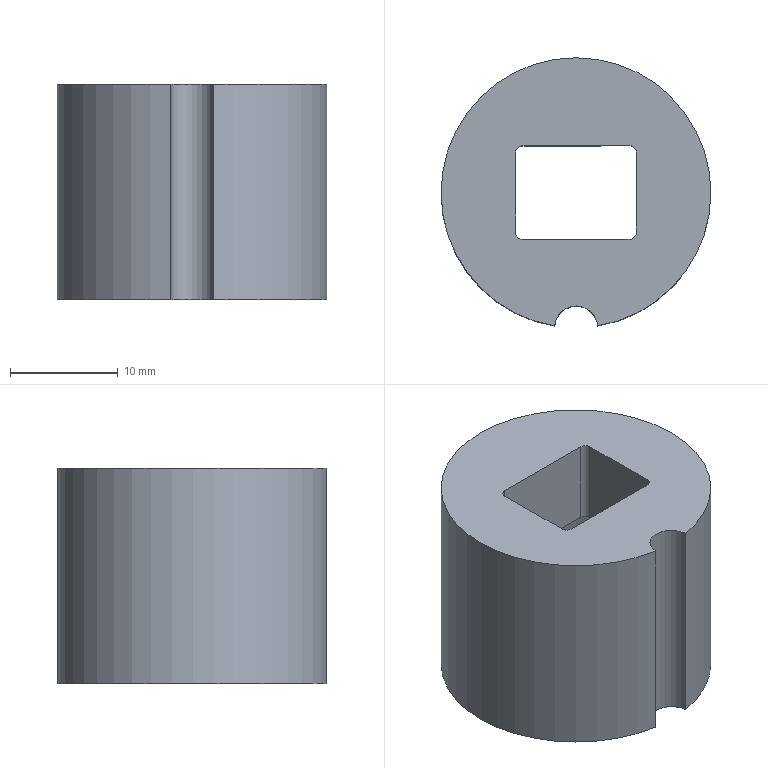Part | NX | features solid 2 | 1 solid | 14 faces | box 25 x 24.842 x 20 mm | volume 6327 mm3 | plane 7 | cylinder 7 | commonest cylinder face diameters 1.17 x4 4 x1 16.6 x1 25 x1
STEP:
#1=CARTESIAN_POINT('',(-382.054,-90.843,41.812));
#2=VERTEX_POINT('',#1);
#3=CARTESIAN_POINT('',(-378.067,-90.838,41.812));
#4=VERTEX_POINT('',#3);
#5=CARTESIAN_POINT('',(-380.06,-91.001,41.812));
#6=DIRECTION('',(0.,0.,-1.));
#7=DIRECTION('',(-0.001177,1.,0.));
#8=AXIS2_PLACEMENT_3D('',#5,#6,#7);
#9=CIRCLE('',#8,2.);
#10=EDGE_CURVE('',#2,#4,#9,.T.);
#11=ORIENTED_EDGE('',*,*,#10,.T.);
#12=CARTESIAN_POINT('',(-380.075,-78.501,41.812));
#13=DIRECTION('',(0.,0.,-1.));
#14=DIRECTION('',(-0.001177,1.,0.));
#15=AXIS2_PLACEMENT_3D('',#12,#13,#14);
#16=CIRCLE('',#15,12.5);
#17=EDGE_CURVE('',#2,#4,#16,.T.);
#18=ORIENTED_EDGE('',*,*,#17,.F.);
#19=EDGE_LOOP('',(#11,#18));
#20=FACE_BOUND('',#19,.T.);
#21=CARTESIAN_POINT('',(-375.07,-82.83,41.812));
#22=VERTEX_POINT('',#21);
#23=CARTESIAN_POINT('',(-374.485,-82.244,41.812));
#24=VERTEX_POINT('',#23);
#25=CARTESIAN_POINT('',(-375.07,-82.245,41.812));
#26=DIRECTION('',(0.,0.,1.));
#27=DIRECTION('',(1.,0.,0.));
#28=AXIS2_PLACEMENT_3D('',#25,#26,#27);
#29=CIRCLE('',#28,0.585);
#30=EDGE_CURVE('',#22,#24,#29,.T.);
#31=ORIENTED_EDGE('',*,*,#30,.F.);
#32=CARTESIAN_POINT('',(-385.07,-82.841,41.812));
#33=VERTEX_POINT('',#32);
#34=CARTESIAN_POINT('',(-380.07,-82.836,41.812));
#35=DIRECTION('',(-1.,-0.001177,0.));
#36=VECTOR('',#35,1000.);
#37=LINE('',#34,#36);
#38=EDGE_CURVE('',#22,#33,#37,.T.);
#39=ORIENTED_EDGE('',*,*,#38,.T.);
#40=CARTESIAN_POINT('',(-385.655,-82.257,41.812));
#41=VERTEX_POINT('',#40);
#42=CARTESIAN_POINT('',(-385.07,-82.256,41.812));
#43=DIRECTION('',(0.,0.,1.));
#44=DIRECTION('',(1.,0.,0.));
#45=AXIS2_PLACEMENT_3D('',#42,#43,#44);
#46=CIRCLE('',#45,0.585);
#47=EDGE_CURVE('',#41,#33,#46,.T.);
#48=ORIENTED_EDGE('',*,*,#47,.F.);
#49=CARTESIAN_POINT('',(-385.664,-74.757,41.812));
#50=VERTEX_POINT('',#49);
#51=CARTESIAN_POINT('',(-385.66,-78.507,41.812));
#52=DIRECTION('',(-0.001177,1.,0.));
#53=VECTOR('',#52,1000.);
#54=LINE('',#51,#53);
#55=EDGE_CURVE('',#41,#50,#54,.T.);
#56=ORIENTED_EDGE('',*,*,#55,.T.);
#57=CARTESIAN_POINT('',(-385.08,-74.171,41.812));
#58=VERTEX_POINT('',#57);
#59=CARTESIAN_POINT('',(-385.079,-74.756,41.812));
#60=DIRECTION('',(0.,0.,1.));
#61=DIRECTION('',(1.,0.,0.));
#62=AXIS2_PLACEMENT_3D('',#59,#60,#61);
#63=CIRCLE('',#62,0.585);
#64=EDGE_CURVE('',#58,#50,#63,.T.);
#65=ORIENTED_EDGE('',*,*,#64,.F.);
#66=CARTESIAN_POINT('',(-375.08,-74.16,41.812));
#67=VERTEX_POINT('',#66);
#68=CARTESIAN_POINT('',(-380.08,-74.166,41.812));
#69=DIRECTION('',(1.,0.001177,0.));
#70=VECTOR('',#69,1000.);
#71=LINE('',#68,#70);
#72=EDGE_CURVE('',#58,#67,#71,.T.);
#73=ORIENTED_EDGE('',*,*,#72,.T.);
#74=CARTESIAN_POINT('',(-374.494,-74.744,41.812));
#75=VERTEX_POINT('',#74);
#76=CARTESIAN_POINT('',(-375.079,-74.745,41.812));
#77=DIRECTION('',(0.,0.,1.));
#78=DIRECTION('',(1.,0.,0.));
#79=AXIS2_PLACEMENT_3D('',#76,#77,#78);
#80=CIRCLE('',#79,0.585);
#81=EDGE_CURVE('',#75,#67,#80,.T.);
#82=ORIENTED_EDGE('',*,*,#81,.F.);
#83=CARTESIAN_POINT('',(-374.49,-78.494,41.812));
#84=DIRECTION('',(0.001177,-1.,0.));
#85=VECTOR('',#84,1000.);
#86=LINE('',#83,#85);
#87=EDGE_CURVE('',#75,#24,#86,.T.);
#88=ORIENTED_EDGE('',*,*,#87,.T.);
#89=EDGE_LOOP('',(#31,#39,#48,#56,#65,#73,#82,#88));
#90=FACE_BOUND('',#89,.T.);
#91=CARTESIAN_POINT('',(-380.075,-78.501,41.812));
#92=DIRECTION('',(0.,0.,1.));
#93=DIRECTION('',(0.001177,-1.,0.));
#94=AXIS2_PLACEMENT_3D('',#91,#92,#93);
#95=PLANE('',#94);
#96=ADVANCED_FACE('',(#20,#90),#95,.T.);
#97=CARTESIAN_POINT('',(-378.067,-90.838,21.812));
#98=VERTEX_POINT('',#97);
#99=CARTESIAN_POINT('',(-382.054,-90.843,21.812));
#100=VERTEX_POINT('',#99);
#101=CARTESIAN_POINT('',(-380.06,-91.001,21.812));
#102=DIRECTION('',(0.,0.,1.));
#103=DIRECTION('',(0.001177,-1.,0.));
#104=AXIS2_PLACEMENT_3D('',#101,#102,#103);
#105=CIRCLE('',#104,2.);
#106=EDGE_CURVE('',#98,#100,#105,.T.);
#107=ORIENTED_EDGE('',*,*,#106,.T.);
#108=CARTESIAN_POINT('',(-380.075,-78.501,21.812));
#109=DIRECTION('',(0.,0.,1.));
#110=DIRECTION('',(0.001177,-1.,0.));
#111=AXIS2_PLACEMENT_3D('',#108,#109,#110);
#112=CIRCLE('',#111,12.5);
#113=EDGE_CURVE('',#98,#100,#112,.T.);
#114=ORIENTED_EDGE('',*,*,#113,.F.);
#115=EDGE_LOOP('',(#107,#114));
#116=FACE_BOUND('',#115,.T.);
#117=CARTESIAN_POINT('',(-380.065,-86.801,21.812));
#118=VERTEX_POINT('',#117);
#119=CARTESIAN_POINT('',(-380.075,-78.501,21.812));
#120=DIRECTION('',(0.,0.,1.));
#121=DIRECTION('',(0.001177,-1.,0.));
#122=AXIS2_PLACEMENT_3D('',#119,#120,#121);
#123=CIRCLE('',#122,8.3);
#124=EDGE_CURVE('',#118,#118,#123,.T.);
#125=ORIENTED_EDGE('',*,*,#124,.T.);
#126=EDGE_LOOP('',(#125));
#127=FACE_BOUND('',#126,.T.);
#128=CARTESIAN_POINT('',(-380.075,-78.501,21.812));
#129=DIRECTION('',(0.,0.,-1.));
#130=DIRECTION('',(-0.001177,1.,0.));
#131=AXIS2_PLACEMENT_3D('',#128,#129,#130);
#132=PLANE('',#131);
#133=ADVANCED_FACE('',(#116,#127),#132,.T.);
#134=CARTESIAN_POINT('',(-378.067,-90.838,31.812));
#135=DIRECTION('',(0.,0.,1.));
#136=VECTOR('',#135,1000.);
#137=LINE('',#134,#136);
#138=EDGE_CURVE('',#98,#4,#137,.T.);
#139=ORIENTED_EDGE('',*,*,#138,.F.);
#140=ORIENTED_EDGE('',*,*,#113,.T.);
#141=CARTESIAN_POINT('',(-382.054,-90.843,31.812));
#142=DIRECTION('',(0.,0.,1.));
#143=VECTOR('',#142,1000.);
#144=LINE('',#141,#143);
#145=EDGE_CURVE('',#2,#100,#144,.F.);
#146=ORIENTED_EDGE('',*,*,#145,.F.);
#147=ORIENTED_EDGE('',*,*,#17,.T.);
#148=EDGE_LOOP('',(#139,#140,#146,#147));
#149=FACE_BOUND('',#148,.T.);
#150=CARTESIAN_POINT('',(-380.075,-78.501,21.812));
#151=DIRECTION('',(0.,0.,1.));
#152=DIRECTION('',(0.001177,-1.,0.));
#153=AXIS2_PLACEMENT_3D('',#150,#151,#152);
#154=CYLINDRICAL_SURFACE('',#153,12.5);
#155=ADVANCED_FACE('',(#149),#154,.T.);
#156=CARTESIAN_POINT('',(-385.07,-82.841,33.812));
#157=VERTEX_POINT('',#156);
#158=CARTESIAN_POINT('',(-375.07,-82.83,33.812));
#159=VERTEX_POINT('',#158);
#160=CARTESIAN_POINT('',(-380.07,-82.836,33.812));
#161=DIRECTION('',(1.,0.001177,0.));
#162=VECTOR('',#161,1000.);
#163=LINE('',#160,#162);
#164=EDGE_CURVE('',#157,#159,#163,.T.);
#165=ORIENTED_EDGE('',*,*,#164,.T.);
#166=CARTESIAN_POINT('',(-374.485,-82.244,33.812));
#167=VERTEX_POINT('',#166);
#168=CARTESIAN_POINT('',(-375.07,-82.245,33.812));
#169=DIRECTION('',(0.,0.,-1.));
#170=DIRECTION('',(-1.,0.,0.));
#171=AXIS2_PLACEMENT_3D('',#168,#169,#170);
#172=CIRCLE('',#171,0.585);
#173=EDGE_CURVE('',#167,#159,#172,.T.);
#174=ORIENTED_EDGE('',*,*,#173,.F.);
#175=CARTESIAN_POINT('',(-374.494,-74.744,33.812));
#176=VERTEX_POINT('',#175);
#177=CARTESIAN_POINT('',(-374.49,-78.494,33.812));
#178=DIRECTION('',(-0.001177,1.,0.));
#179=VECTOR('',#178,1000.);
#180=LINE('',#177,#179);
#181=EDGE_CURVE('',#167,#176,#180,.T.);
#182=ORIENTED_EDGE('',*,*,#181,.T.);
#183=CARTESIAN_POINT('',(-375.08,-74.16,33.812));
#184=VERTEX_POINT('',#183);
#185=CARTESIAN_POINT('',(-375.079,-74.745,33.812));
#186=DIRECTION('',(0.,0.,-1.));
#187=DIRECTION('',(-1.,0.,0.));
#188=AXIS2_PLACEMENT_3D('',#185,#186,#187);
#189=CIRCLE('',#188,0.585);
#190=EDGE_CURVE('',#184,#176,#189,.T.);
#191=ORIENTED_EDGE('',*,*,#190,.F.);
#192=CARTESIAN_POINT('',(-385.08,-74.171,33.812));
#193=VERTEX_POINT('',#192);
#194=CARTESIAN_POINT('',(-380.08,-74.166,33.812));
#195=DIRECTION('',(-1.,-0.001177,0.));
#196=VECTOR('',#195,1000.);
#197=LINE('',#194,#196);
#198=EDGE_CURVE('',#184,#193,#197,.T.);
#199=ORIENTED_EDGE('',*,*,#198,.T.);
#200=CARTESIAN_POINT('',(-385.664,-74.757,33.812));
#201=VERTEX_POINT('',#200);
#202=CARTESIAN_POINT('',(-385.079,-74.756,33.812));
#203=DIRECTION('',(0.,0.,-1.));
#204=DIRECTION('',(-1.,0.,0.));
#205=AXIS2_PLACEMENT_3D('',#202,#203,#204);
#206=CIRCLE('',#205,0.585);
#207=EDGE_CURVE('',#201,#193,#206,.T.);
#208=ORIENTED_EDGE('',*,*,#207,.F.);
#209=CARTESIAN_POINT('',(-385.655,-82.257,33.812));
#210=VERTEX_POINT('',#209);
#211=CARTESIAN_POINT('',(-385.66,-78.507,33.812));
#212=DIRECTION('',(0.001177,-1.,0.));
#213=VECTOR('',#212,1000.);
#214=LINE('',#211,#213);
#215=EDGE_CURVE('',#201,#210,#214,.T.);
#216=ORIENTED_EDGE('',*,*,#215,.T.);
#217=CARTESIAN_POINT('',(-385.07,-82.256,33.812));
#218=DIRECTION('',(0.,0.,-1.));
#219=DIRECTION('',(-1.,0.,0.));
#220=AXIS2_PLACEMENT_3D('',#217,#218,#219);
#221=CIRCLE('',#220,0.585);
#222=EDGE_CURVE('',#157,#210,#221,.T.);
#223=ORIENTED_EDGE('',*,*,#222,.F.);
#224=EDGE_LOOP('',(#165,#174,#182,#191,#199,#208,#216,#223));
#225=FACE_BOUND('',#224,.T.);
#226=CARTESIAN_POINT('',(-380.085,-70.201,33.812));
#227=VERTEX_POINT('',#226);
#228=CARTESIAN_POINT('',(-380.075,-78.501,33.812));
#229=DIRECTION('',(0.,0.,-1.));
#230=DIRECTION('',(-0.001177,1.,0.));
#231=AXIS2_PLACEMENT_3D('',#228,#229,#230);
#232=CIRCLE('',#231,8.3);
#233=EDGE_CURVE('',#227,#227,#232,.T.);
#234=ORIENTED_EDGE('',*,*,#233,.T.);
#235=EDGE_LOOP('',(#234));
#236=FACE_BOUND('',#235,.T.);
#237=CARTESIAN_POINT('',(-380.075,-78.501,33.812));
#238=DIRECTION('',(0.,0.,1.));
#239=DIRECTION('',(0.001177,-1.,0.));
#240=AXIS2_PLACEMENT_3D('',#237,#238,#239);
#241=PLANE('',#240);
#242=ADVANCED_FACE('',(#225,#236),#241,.F.);
#243=ORIENTED_EDGE('',*,*,#233,.F.);
#244=EDGE_LOOP('',(#243));
#245=FACE_BOUND('',#244,.T.);
#246=ORIENTED_EDGE('',*,*,#124,.F.);
#247=EDGE_LOOP('',(#246));
#248=FACE_BOUND('',#247,.T.);
#249=CARTESIAN_POINT('',(-380.075,-78.501,21.812));
#250=DIRECTION('',(0.,0.,1.));
#251=DIRECTION('',(0.001177,-1.,0.));
#252=AXIS2_PLACEMENT_3D('',#249,#250,#251);
#253=CYLINDRICAL_SURFACE('',#252,8.3);
#254=ADVANCED_FACE('',(#245,#248),#253,.F.);
#255=ORIENTED_EDGE('',*,*,#215,.F.);
#256=CARTESIAN_POINT('',(-385.664,-74.757,33.812));
#257=DIRECTION('',(0.,0.,1.));
#258=VECTOR('',#257,1000.);
#259=LINE('',#256,#258);
#260=EDGE_CURVE('',#50,#201,#259,.F.);
#261=ORIENTED_EDGE('',*,*,#260,.F.);
#262=ORIENTED_EDGE('',*,*,#55,.F.);
#263=CARTESIAN_POINT('',(-385.655,-82.257,33.812));
#264=DIRECTION('',(0.,0.,1.));
#265=VECTOR('',#264,1000.);
#266=LINE('',#263,#265);
#267=EDGE_CURVE('',#210,#41,#266,.T.);
#268=ORIENTED_EDGE('',*,*,#267,.F.);
#269=EDGE_LOOP('',(#255,#261,#262,#268));
#270=FACE_BOUND('',#269,.T.);
#271=CARTESIAN_POINT('',(-385.66,-78.507,33.812));
#272=DIRECTION('',(-1.,-0.001177,0.));
#273=DIRECTION('',(0.,0.,-1.));
#274=AXIS2_PLACEMENT_3D('',#271,#272,#273);
#275=PLANE('',#274);
#276=ADVANCED_FACE('',(#270),#275,.F.);
#277=ORIENTED_EDGE('',*,*,#72,.F.);
#278=CARTESIAN_POINT('',(-385.08,-74.171,33.812));
#279=DIRECTION('',(0.,0.,1.));
#280=VECTOR('',#279,1000.);
#281=LINE('',#278,#280);
#282=EDGE_CURVE('',#193,#58,#281,.T.);
#283=ORIENTED_EDGE('',*,*,#282,.F.);
#284=ORIENTED_EDGE('',*,*,#198,.F.);
#285=CARTESIAN_POINT('',(-375.08,-74.16,33.812));
#286=DIRECTION('',(0.,0.,1.));
#287=VECTOR('',#286,1000.);
#288=LINE('',#285,#287);
#289=EDGE_CURVE('',#67,#184,#288,.F.);
#290=ORIENTED_EDGE('',*,*,#289,.F.);
#291=EDGE_LOOP('',(#277,#283,#284,#290));
#292=FACE_BOUND('',#291,.T.);
#293=CARTESIAN_POINT('',(-380.08,-74.166,33.812));
#294=DIRECTION('',(-0.001177,1.,0.));
#295=DIRECTION('',(0.,0.,1.));
#296=AXIS2_PLACEMENT_3D('',#293,#294,#295);
#297=PLANE('',#296);
#298=ADVANCED_FACE('',(#292),#297,.F.);
#299=ORIENTED_EDGE('',*,*,#87,.F.);
#300=CARTESIAN_POINT('',(-374.494,-74.744,33.812));
#301=DIRECTION('',(0.,0.,1.));
#302=VECTOR('',#301,1000.);
#303=LINE('',#300,#302);
#304=EDGE_CURVE('',#176,#75,#303,.T.);
#305=ORIENTED_EDGE('',*,*,#304,.F.);
#306=ORIENTED_EDGE('',*,*,#181,.F.);
#307=CARTESIAN_POINT('',(-374.485,-82.244,33.812));
#308=DIRECTION('',(0.,0.,1.));
#309=VECTOR('',#308,1000.);
#310=LINE('',#307,#309);
#311=EDGE_CURVE('',#24,#167,#310,.F.);
#312=ORIENTED_EDGE('',*,*,#311,.F.);
#313=EDGE_LOOP('',(#299,#305,#306,#312));
#314=FACE_BOUND('',#313,.T.);
#315=CARTESIAN_POINT('',(-374.49,-78.494,33.812));
#316=DIRECTION('',(1.,0.001177,0.));
#317=DIRECTION('',(0.,0.,1.));
#318=AXIS2_PLACEMENT_3D('',#315,#316,#317);
#319=PLANE('',#318);
#320=ADVANCED_FACE('',(#314),#319,.F.);
#321=ORIENTED_EDGE('',*,*,#38,.F.);
#322=CARTESIAN_POINT('',(-375.07,-82.83,33.812));
#323=DIRECTION('',(0.,0.,1.));
#324=VECTOR('',#323,1000.);
#325=LINE('',#322,#324);
#326=EDGE_CURVE('',#159,#22,#325,.T.);
#327=ORIENTED_EDGE('',*,*,#326,.F.);
#328=ORIENTED_EDGE('',*,*,#164,.F.);
#329=CARTESIAN_POINT('',(-385.07,-82.841,33.812));
#330=DIRECTION('',(0.,0.,1.));
#331=VECTOR('',#330,1000.);
#332=LINE('',#329,#331);
#333=EDGE_CURVE('',#33,#157,#332,.F.);
#334=ORIENTED_EDGE('',*,*,#333,.F.);
#335=EDGE_LOOP('',(#321,#327,#328,#334));
#336=FACE_BOUND('',#335,.T.);
#337=CARTESIAN_POINT('',(-380.07,-82.836,33.812));
#338=DIRECTION('',(0.001177,-1.,0.));
#339=DIRECTION('',(0.,0.,-1.));
#340=AXIS2_PLACEMENT_3D('',#337,#338,#339);
#341=PLANE('',#340);
#342=ADVANCED_FACE('',(#336),#341,.F.);
#343=ORIENTED_EDGE('',*,*,#222,.T.);
#344=ORIENTED_EDGE('',*,*,#267,.T.);
#345=ORIENTED_EDGE('',*,*,#47,.T.);
#346=ORIENTED_EDGE('',*,*,#333,.T.);
#347=EDGE_LOOP('',(#343,#344,#345,#346));
#348=FACE_BOUND('',#347,.T.);
#349=CARTESIAN_POINT('',(-385.07,-82.256,33.812));
#350=DIRECTION('',(0.,0.,1.));
#351=DIRECTION('',(1.,0.,0.));
#352=AXIS2_PLACEMENT_3D('',#349,#350,#351);
#353=CYLINDRICAL_SURFACE('',#352,0.585);
#354=ADVANCED_FACE('',(#348),#353,.F.);
#355=ORIENTED_EDGE('',*,*,#173,.T.);
#356=ORIENTED_EDGE('',*,*,#326,.T.);
#357=ORIENTED_EDGE('',*,*,#30,.T.);
#358=ORIENTED_EDGE('',*,*,#311,.T.);
#359=EDGE_LOOP('',(#355,#356,#357,#358));
#360=FACE_BOUND('',#359,.T.);
#361=CARTESIAN_POINT('',(-375.07,-82.245,33.812));
#362=DIRECTION('',(0.,0.,1.));
#363=DIRECTION('',(1.,0.,0.));
#364=AXIS2_PLACEMENT_3D('',#361,#362,#363);
#365=CYLINDRICAL_SURFACE('',#364,0.585);
#366=ADVANCED_FACE('',(#360),#365,.F.);
#367=ORIENTED_EDGE('',*,*,#190,.T.);
#368=ORIENTED_EDGE('',*,*,#304,.T.);
#369=ORIENTED_EDGE('',*,*,#81,.T.);
#370=ORIENTED_EDGE('',*,*,#289,.T.);
#371=EDGE_LOOP('',(#367,#368,#369,#370));
#372=FACE_BOUND('',#371,.T.);
#373=CARTESIAN_POINT('',(-375.079,-74.745,33.812));
#374=DIRECTION('',(0.,0.,1.));
#375=DIRECTION('',(1.,0.,0.));
#376=AXIS2_PLACEMENT_3D('',#373,#374,#375);
#377=CYLINDRICAL_SURFACE('',#376,0.585);
#378=ADVANCED_FACE('',(#372),#377,.F.);
#379=ORIENTED_EDGE('',*,*,#207,.T.);
#380=ORIENTED_EDGE('',*,*,#282,.T.);
#381=ORIENTED_EDGE('',*,*,#64,.T.);
#382=ORIENTED_EDGE('',*,*,#260,.T.);
#383=EDGE_LOOP('',(#379,#380,#381,#382));
#384=FACE_BOUND('',#383,.T.);
#385=CARTESIAN_POINT('',(-385.079,-74.756,33.812));
#386=DIRECTION('',(0.,0.,1.));
#387=DIRECTION('',(1.,0.,0.));
#388=AXIS2_PLACEMENT_3D('',#385,#386,#387);
#389=CYLINDRICAL_SURFACE('',#388,0.585);
#390=ADVANCED_FACE('',(#384),#389,.F.);
#391=ORIENTED_EDGE('',*,*,#138,.T.);
#392=ORIENTED_EDGE('',*,*,#10,.F.);
#393=ORIENTED_EDGE('',*,*,#145,.T.);
#394=ORIENTED_EDGE('',*,*,#106,.F.);
#395=EDGE_LOOP('',(#391,#392,#393,#394));
#396=FACE_BOUND('',#395,.T.);
#397=CARTESIAN_POINT('',(-380.06,-91.001,21.812));
#398=DIRECTION('',(0.,0.,1.));
#399=DIRECTION('',(0.001177,-1.,0.));
#400=AXIS2_PLACEMENT_3D('',#397,#398,#399);
#401=CYLINDRICAL_SURFACE('',#400,2.);
#402=ADVANCED_FACE('',(#396),#401,.F.);
#403=CLOSED_SHELL('',(#96,#133,#155,#242,#254,#276,#298,#320,#342,#354,#366,#378,#390,#402));
#404=MANIFOLD_SOLID_BREP('',#403);
#405=(LENGTH_UNIT()NAMED_UNIT(*)SI_UNIT(.MILLI.,.METRE.));
#406=UNCERTAINTY_MEASURE_WITH_UNIT(LENGTH_MEASURE(0.00001),#405,'','');
#407=(NAMED_UNIT(*)PLANE_ANGLE_UNIT()SI_UNIT($,.RADIAN.));
#408=(NAMED_UNIT(*)SI_UNIT($,.STERADIAN.)SOLID_ANGLE_UNIT());
#409=(GEOMETRIC_REPRESENTATION_CONTEXT(3)GLOBAL_UNCERTAINTY_ASSIGNED_CONTEXT((#406))GLOBAL_UNIT_ASSIGNED_CONTEXT((#405,#407,#408))REPRESENTATION_CONTEXT('',''));
#410=ADVANCED_BREP_SHAPE_REPRESENTATION('',(#404),#409);